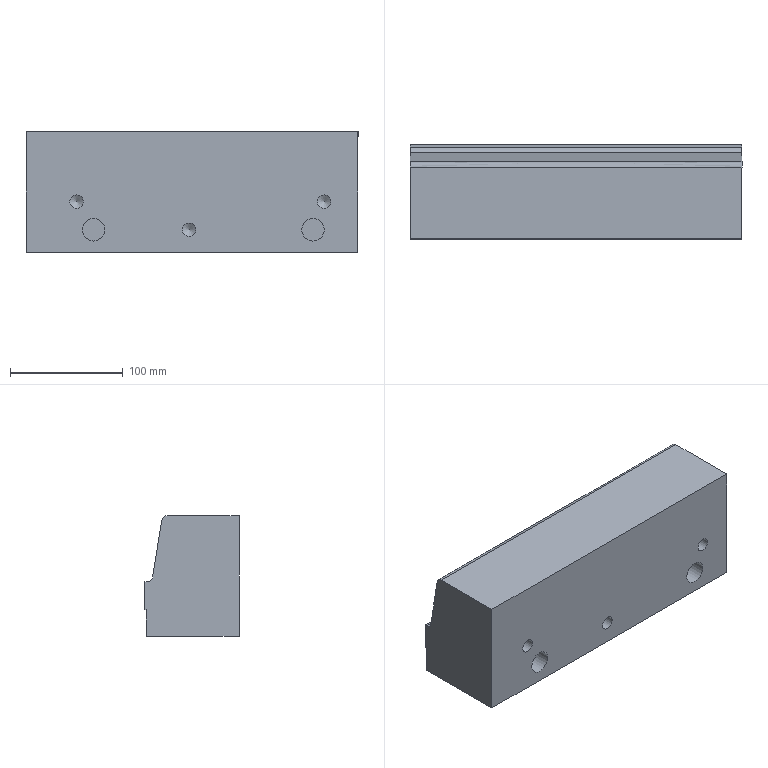Part | NX | features solid 2 | 1 solid | 22 faces | box 295 x 83.706 x 107.133 mm | volume 2418413 mm3 | plane 9 | cylinder 6 | spline 4 | cone 3 | commonest cylinder face diameters 12 x3 20 x2 10 x1
STEP:
#1=CARTESIAN_POINT('',(75.,-77.708,-50.));
#2=VERTEX_POINT('',#1);
#3=CARTESIAN_POINT('',(370.,-77.709,-50.));
#4=VERTEX_POINT('',#3);
#5=CARTESIAN_POINT('',(75.,-77.708,-50.));
#6=CARTESIAN_POINT('',(173.333,-77.71,-50.));
#7=CARTESIAN_POINT('',(271.667,-77.709,-50.));
#8=CARTESIAN_POINT('',(370.,-77.709,-50.));
#9=B_SPLINE_CURVE_WITH_KNOTS('',3,(#5,#6,#7,#8),.UNSPECIFIED.,.F.,.F.,(4,4),(0.1723,0.4673),.UNSPECIFIED.);
#10=EDGE_CURVE('',#2,#4,#9,.T.);
#11=ORIENTED_EDGE('',*,*,#10,.F.);
#12=CARTESIAN_POINT('',(75.,-77.507,-26.5));
#13=VERTEX_POINT('',#12);
#14=CARTESIAN_POINT('',(75.,-77.608,-38.267));
#15=DIRECTION('',(0.,-0.008536,-1.));
#16=VECTOR('',#15,1000.);
#17=LINE('',#14,#16);
#18=EDGE_CURVE('',#2,#13,#17,.F.);
#19=ORIENTED_EDGE('',*,*,#18,.T.);
#20=CARTESIAN_POINT('',(370.,-77.508,-26.5));
#21=VERTEX_POINT('',#20);
#22=CARTESIAN_POINT('',(75.,-77.507,-26.5));
#23=CARTESIAN_POINT('',(173.333,-77.509,-26.5));
#24=CARTESIAN_POINT('',(271.667,-77.508,-26.5));
#25=CARTESIAN_POINT('',(370.,-77.508,-26.5));
#26=B_SPLINE_CURVE_WITH_KNOTS('',3,(#22,#23,#24,#25),.UNSPECIFIED.,.F.,.F.,(4,4),(0.1378,0.4328),.UNSPECIFIED.);
#27=EDGE_CURVE('',#13,#21,#26,.T.);
#28=ORIENTED_EDGE('',*,*,#27,.T.);
#29=CARTESIAN_POINT('',(370.,-77.608,-38.267));
#30=DIRECTION('',(0.,-0.008536,-1.));
#31=VECTOR('',#30,1000.);
#32=LINE('',#29,#31);
#33=EDGE_CURVE('',#4,#21,#32,.F.);
#34=ORIENTED_EDGE('',*,*,#33,.F.);
#35=EDGE_LOOP('',(#11,#19,#28,#34));
#36=FACE_BOUND('',#35,.T.);
#37=CARTESIAN_POINT('',(75.,-77.507,-26.5));
#38=CARTESIAN_POINT('',(75.,-77.708,-50.));
#39=CARTESIAN_POINT('',(173.333,-77.509,-26.5));
#40=CARTESIAN_POINT('',(173.333,-77.71,-50.));
#41=CARTESIAN_POINT('',(271.667,-77.508,-26.5));
#42=CARTESIAN_POINT('',(271.667,-77.709,-50.));
#43=CARTESIAN_POINT('',(370.,-77.508,-26.5));
#44=CARTESIAN_POINT('',(370.,-77.709,-50.));
#45=B_SPLINE_SURFACE_WITH_KNOTS('',3,1,((#37,#38),(#39,#40),(#41,#42),(#43,#44)),.SURF_OF_LINEAR_EXTRUSION.,.F.,.F.,.F.,(4,4),(2,2),(0.5716,0.7876),(0.,1.),.PIECEWISE_BEZIER_KNOTS.);
#46=ADVANCED_FACE('',(#36),#45,.T.);
#47=ORIENTED_EDGE('',*,*,#33,.T.);
#48=CARTESIAN_POINT('',(370.,-76.295,-26.51));
#49=VERTEX_POINT('',#48);
#50=CARTESIAN_POINT('',(370.,-76.914,-26.505));
#51=DIRECTION('',(0.,-1.,0.008536));
#52=VECTOR('',#51,1000.);
#53=LINE('',#50,#52);
#54=EDGE_CURVE('',#49,#21,#53,.T.);
#55=ORIENTED_EDGE('',*,*,#54,.F.);
#56=CARTESIAN_POINT('',(370.,-76.295,-1.509));
#57=VERTEX_POINT('',#56);
#58=CARTESIAN_POINT('',(370.,-76.295,-14.009));
#59=DIRECTION('',(0.,0.,-1.));
#60=VECTOR('',#59,1000.);
#61=LINE('',#58,#60);
#62=EDGE_CURVE('',#57,#49,#61,.T.);
#63=ORIENTED_EDGE('',*,*,#62,.F.);
#64=CARTESIAN_POINT('',(370.,-78.294,-1.492));
#65=VERTEX_POINT('',#64);
#66=CARTESIAN_POINT('',(370.,46.797,-2.56));
#67=DIRECTION('',(0.,1.,-0.008536));
#68=VECTOR('',#67,1000.);
#69=LINE('',#66,#68);
#70=EDGE_CURVE('',#65,#57,#69,.T.);
#71=ORIENTED_EDGE('',*,*,#70,.F.);
#72=CARTESIAN_POINT('',(370.,-83.189,2.72));
#73=VERTEX_POINT('',#72);
#74=CARTESIAN_POINT('',(370.,-78.252,3.508));
#75=DIRECTION('',(-1.,0.,0.));
#76=DIRECTION('',(0.,0.,1.));
#77=AXIS2_PLACEMENT_3D('',#74,#75,#76);
#78=CIRCLE('',#77,5.);
#79=EDGE_CURVE('',#73,#65,#78,.F.);
#80=ORIENTED_EDGE('',*,*,#79,.F.);
#81=CARTESIAN_POINT('',(370.,-91.197,52.92));
#82=VERTEX_POINT('',#81);
#83=CARTESIAN_POINT('',(370.,-87.499,29.736));
#84=DIRECTION('',(0.,0.1575,-0.9875));
#85=VECTOR('',#84,1000.);
#86=LINE('',#83,#85);
#87=EDGE_CURVE('',#82,#73,#86,.T.);
#88=ORIENTED_EDGE('',*,*,#87,.F.);
#89=CARTESIAN_POINT('',(370.,-96.134,57.133));
#90=VERTEX_POINT('',#89);
#91=CARTESIAN_POINT('',(370.,-96.134,52.133));
#92=DIRECTION('',(-1.,0.,0.));
#93=DIRECTION('',(0.,0.,1.));
#94=AXIS2_PLACEMENT_3D('',#91,#92,#93);
#95=CIRCLE('',#94,5.);
#96=EDGE_CURVE('',#82,#90,#95,.F.);
#97=ORIENTED_EDGE('',*,*,#96,.T.);
#98=CARTESIAN_POINT('',(370.,-160.,57.133));
#99=VERTEX_POINT('',#98);
#100=CARTESIAN_POINT('',(370.,-91.869,57.133));
#101=DIRECTION('',(0.,-1.,0.));
#102=VECTOR('',#101,1000.);
#103=LINE('',#100,#102);
#104=EDGE_CURVE('',#90,#99,#103,.T.);
#105=ORIENTED_EDGE('',*,*,#104,.T.);
#106=CARTESIAN_POINT('',(370.,-160.,-50.));
#107=VERTEX_POINT('',#106);
#108=CARTESIAN_POINT('',(370.,-160.,200.));
#109=DIRECTION('',(0.,0.,1.));
#110=VECTOR('',#109,1000.);
#111=LINE('',#108,#110);
#112=EDGE_CURVE('',#107,#99,#111,.T.);
#113=ORIENTED_EDGE('',*,*,#112,.F.);
#114=CARTESIAN_POINT('',(370.,360.,-50.));
#115=DIRECTION('',(0.,-1.,0.));
#116=VECTOR('',#115,1000.);
#117=LINE('',#114,#116);
#118=EDGE_CURVE('',#107,#4,#117,.F.);
#119=ORIENTED_EDGE('',*,*,#118,.T.);
#120=EDGE_LOOP('',(#47,#55,#63,#71,#80,#88,#97,#105,#113,#119));
#121=FACE_BOUND('',#120,.T.);
#122=CARTESIAN_POINT('',(370.,360.,0.));
#123=DIRECTION('',(-1.,0.,0.));
#124=DIRECTION('',(0.,0.,1.));
#125=AXIS2_PLACEMENT_3D('',#122,#123,#124);
#126=PLANE('',#125);
#127=ADVANCED_FACE('',(#121),#126,.F.);
#128=CARTESIAN_POINT('',(75.,-160.,-50.));
#129=VERTEX_POINT('',#128);
#130=CARTESIAN_POINT('',(75.,-160.,-50.));
#131=DIRECTION('',(0.,1.,0.));
#132=VECTOR('',#131,1000.);
#133=LINE('',#130,#132);
#134=EDGE_CURVE('',#129,#2,#133,.T.);
#135=ORIENTED_EDGE('',*,*,#134,.T.);
#136=ORIENTED_EDGE('',*,*,#10,.T.);
#137=ORIENTED_EDGE('',*,*,#118,.F.);
#138=CARTESIAN_POINT('',(-571.479,-160.,-50.));
#139=DIRECTION('',(1.,0.,0.));
#140=VECTOR('',#139,1000.);
#141=LINE('',#138,#140);
#142=EDGE_CURVE('',#129,#107,#141,.T.);
#143=ORIENTED_EDGE('',*,*,#142,.F.);
#144=EDGE_LOOP('',(#135,#136,#137,#143));
#145=FACE_BOUND('',#144,.T.);
#146=CARTESIAN_POINT('',(-571.479,-75.471,-50.));
#147=DIRECTION('',(0.,0.,-1.));
#148=DIRECTION('',(-1.,0.,0.));
#149=AXIS2_PLACEMENT_3D('',#146,#147,#148);
#150=PLANE('',#149);
#151=ADVANCED_FACE('',(#145),#150,.T.);
#152=ORIENTED_EDGE('',*,*,#142,.T.);
#153=ORIENTED_EDGE('',*,*,#112,.T.);
#154=CARTESIAN_POINT('',(75.,-160.,57.133));
#155=VERTEX_POINT('',#154);
#156=CARTESIAN_POINT('',(-705.,-160.,57.133));
#157=DIRECTION('',(1.,0.,0.));
#158=VECTOR('',#157,1000.);
#159=LINE('',#156,#158);
#160=EDGE_CURVE('',#155,#99,#159,.T.);
#161=ORIENTED_EDGE('',*,*,#160,.F.);
#162=CARTESIAN_POINT('',(75.,-160.,200.));
#163=DIRECTION('',(0.,0.,1.));
#164=VECTOR('',#163,1000.);
#165=LINE('',#162,#164);
#166=EDGE_CURVE('',#129,#155,#165,.T.);
#167=ORIENTED_EDGE('',*,*,#166,.F.);
#168=EDGE_LOOP('',(#152,#153,#161,#167));
#169=FACE_BOUND('',#168,.T.);
#170=CARTESIAN_POINT('',(340.,-160.,1.));
#171=VERTEX_POINT('',#170);
#172=CARTESIAN_POINT('',(340.,-160.,-5.));
#173=DIRECTION('',(0.,1.,0.));
#174=DIRECTION('',(0.,0.,1.));
#175=AXIS2_PLACEMENT_3D('',#172,#173,#174);
#176=CIRCLE('',#175,6.);
#177=EDGE_CURVE('',#171,#171,#176,.T.);
#178=ORIENTED_EDGE('',*,*,#177,.T.);
#179=EDGE_LOOP('',(#178));
#180=FACE_BOUND('',#179,.T.);
#181=CARTESIAN_POINT('',(220.,-160.,-24.));
#182=VERTEX_POINT('',#181);
#183=CARTESIAN_POINT('',(220.,-160.,-30.));
#184=DIRECTION('',(0.,1.,0.));
#185=DIRECTION('',(0.,0.,1.));
#186=AXIS2_PLACEMENT_3D('',#183,#184,#185);
#187=CIRCLE('',#186,6.);
#188=EDGE_CURVE('',#182,#182,#187,.T.);
#189=ORIENTED_EDGE('',*,*,#188,.T.);
#190=EDGE_LOOP('',(#189));
#191=FACE_BOUND('',#190,.T.);
#192=CARTESIAN_POINT('',(120.,-160.,1.));
#193=VERTEX_POINT('',#192);
#194=CARTESIAN_POINT('',(120.,-160.,-5.));
#195=DIRECTION('',(0.,1.,0.));
#196=DIRECTION('',(0.,0.,1.));
#197=AXIS2_PLACEMENT_3D('',#194,#195,#196);
#198=CIRCLE('',#197,6.);
#199=EDGE_CURVE('',#193,#193,#198,.T.);
#200=ORIENTED_EDGE('',*,*,#199,.T.);
#201=EDGE_LOOP('',(#200));
#202=FACE_BOUND('',#201,.T.);
#203=CARTESIAN_POINT('',(330.,-160.,-20.));
#204=VERTEX_POINT('',#203);
#205=CARTESIAN_POINT('',(330.,-160.,-30.));
#206=DIRECTION('',(0.,1.,0.));
#207=DIRECTION('',(0.,0.,1.));
#208=AXIS2_PLACEMENT_3D('',#205,#206,#207);
#209=CIRCLE('',#208,10.);
#210=EDGE_CURVE('',#204,#204,#209,.T.);
#211=ORIENTED_EDGE('',*,*,#210,.T.);
#212=EDGE_LOOP('',(#211));
#213=FACE_BOUND('',#212,.T.);
#214=CARTESIAN_POINT('',(135.,-160.,-20.));
#215=VERTEX_POINT('',#214);
#216=CARTESIAN_POINT('',(135.,-160.,-30.));
#217=DIRECTION('',(0.,1.,0.));
#218=DIRECTION('',(0.,0.,1.));
#219=AXIS2_PLACEMENT_3D('',#216,#217,#218);
#220=CIRCLE('',#219,10.);
#221=EDGE_CURVE('',#215,#215,#220,.T.);
#222=ORIENTED_EDGE('',*,*,#221,.T.);
#223=EDGE_LOOP('',(#222));
#224=FACE_BOUND('',#223,.T.);
#225=CARTESIAN_POINT('',(-705.,-160.,200.));
#226=DIRECTION('',(0.,1.,0.));
#227=DIRECTION('',(0.,0.,1.));
#228=AXIS2_PLACEMENT_3D('',#225,#226,#227);
#229=PLANE('',#228);
#230=ADVANCED_FACE('',(#169,#180,#191,#202,#213,#224),#229,.F.);
#231=ORIENTED_EDGE('',*,*,#96,.F.);
#232=CARTESIAN_POINT('',(75.,-91.197,52.92));
#233=VERTEX_POINT('',#232);
#234=CARTESIAN_POINT('',(75.,-91.197,52.92));
#235=CARTESIAN_POINT('',(173.333,-91.197,52.92));
#236=CARTESIAN_POINT('',(271.667,-91.197,52.92));
#237=CARTESIAN_POINT('',(370.,-91.197,52.92));
#238=B_SPLINE_CURVE_WITH_KNOTS('',3,(#234,#235,#236,#237),.UNSPECIFIED.,.F.,.F.,(4,4),(0.2731,0.5681),.UNSPECIFIED.);
#239=EDGE_CURVE('',#233,#82,#238,.T.);
#240=ORIENTED_EDGE('',*,*,#239,.F.);
#241=CARTESIAN_POINT('',(75.,-96.134,57.133));
#242=VERTEX_POINT('',#241);
#243=CARTESIAN_POINT('',(75.,-96.134,52.133));
#244=DIRECTION('',(-1.,0.,0.));
#245=DIRECTION('',(0.,0.,1.));
#246=AXIS2_PLACEMENT_3D('',#243,#244,#245);
#247=CIRCLE('',#246,5.);
#248=EDGE_CURVE('',#233,#242,#247,.F.);
#249=ORIENTED_EDGE('',*,*,#248,.T.);
#250=CARTESIAN_POINT('',(370.,-96.134,57.133));
#251=CARTESIAN_POINT('',(271.667,-96.134,57.133));
#252=CARTESIAN_POINT('',(173.333,-96.134,57.133));
#253=CARTESIAN_POINT('',(75.,-96.134,57.133));
#254=B_SPLINE_CURVE_WITH_KNOTS('',3,(#250,#251,#252,#253),.UNSPECIFIED.,.F.,.F.,(4,4),(0.3736,0.6686),.UNSPECIFIED.);
#255=EDGE_CURVE('',#90,#242,#254,.T.);
#256=ORIENTED_EDGE('',*,*,#255,.F.);
#257=EDGE_LOOP('',(#231,#240,#249,#256));
#258=FACE_BOUND('',#257,.T.);
#259=CARTESIAN_POINT('',(370.,-91.197,52.92));
#260=CARTESIAN_POINT('',(370.,-91.869,57.133));
#261=CARTESIAN_POINT('',(370.,-96.134,57.133));
#262=CARTESIAN_POINT('',(271.667,-91.197,52.92));
#263=CARTESIAN_POINT('',(271.667,-91.869,57.133));
#264=CARTESIAN_POINT('',(271.667,-96.134,57.133));
#265=CARTESIAN_POINT('',(173.333,-91.197,52.92));
#266=CARTESIAN_POINT('',(173.333,-91.869,57.133));
#267=CARTESIAN_POINT('',(173.333,-96.134,57.133));
#268=CARTESIAN_POINT('',(75.,-91.197,52.92));
#269=CARTESIAN_POINT('',(75.,-91.869,57.133));
#270=CARTESIAN_POINT('',(75.,-96.134,57.133));
#271=(BOUNDED_SURFACE()B_SPLINE_SURFACE(3,2,((#259,#260,#261),(#262,#263,#264),(#265,#266,#267),(#268,#269,#270)),.UNSPECIFIED.,.F.,.F.,.F.)B_SPLINE_SURFACE_WITH_KNOTS((4,4),(3,3),(0.4893,0.7843),(0.,1.),.PIECEWISE_BEZIER_KNOTS.)GEOMETRIC_REPRESENTATION_ITEM()RATIONAL_B_SPLINE_SURFACE(((1.,0.7608,1.),(1.,0.7608,1.),(1.,0.7608,1.),(1.,0.7608,1.)))REPRESENTATION_ITEM('')SURFACE());
#272=ADVANCED_FACE('',(#258),#271,.T.);
#273=ORIENTED_EDGE('',*,*,#239,.T.);
#274=ORIENTED_EDGE('',*,*,#87,.T.);
#275=CARTESIAN_POINT('',(75.,-83.189,2.72));
#276=VERTEX_POINT('',#275);
#277=CARTESIAN_POINT('',(75.,-83.189,2.72));
#278=CARTESIAN_POINT('',(173.333,-83.189,2.72));
#279=CARTESIAN_POINT('',(271.667,-83.189,2.72));
#280=CARTESIAN_POINT('',(370.,-83.189,2.72));
#281=B_SPLINE_CURVE_WITH_KNOTS('',3,(#277,#278,#279,#280),.UNSPECIFIED.,.F.,.F.,(4,4),(0.3113,0.6615),.UNSPECIFIED.);
#282=EDGE_CURVE('',#276,#73,#281,.T.);
#283=ORIENTED_EDGE('',*,*,#282,.F.);
#284=CARTESIAN_POINT('',(75.,-87.499,29.736));
#285=DIRECTION('',(0.,0.1575,-0.9875));
#286=VECTOR('',#285,1000.);
#287=LINE('',#284,#286);
#288=EDGE_CURVE('',#233,#276,#287,.T.);
#289=ORIENTED_EDGE('',*,*,#288,.F.);
#290=EDGE_LOOP('',(#273,#274,#283,#289));
#291=FACE_BOUND('',#290,.T.);
#292=CARTESIAN_POINT('',(808.196,-82.695,-0.3814));
#293=CARTESIAN_POINT('',(-199.284,-82.695,-0.3814));
#294=CARTESIAN_POINT('',(808.196,-92.303,59.853));
#295=CARTESIAN_POINT('',(-199.284,-92.303,59.853));
#296=B_SPLINE_SURFACE_WITH_KNOTS('',1,1,((#292,#293),(#294,#295)),.PLANE_SURF.,.F.,.F.,.F.,(2,2),(2,2),(-0.06964,1.283),(-0.1722,1.),.UNSPECIFIED.);
#297=ADVANCED_FACE('',(#291),#296,.F.);
#298=ORIENTED_EDGE('',*,*,#282,.T.);
#299=ORIENTED_EDGE('',*,*,#79,.T.);
#300=CARTESIAN_POINT('',(75.,-78.294,-1.492));
#301=VERTEX_POINT('',#300);
#302=CARTESIAN_POINT('',(370.,-78.294,-1.492));
#303=CARTESIAN_POINT('',(271.667,-78.294,-1.492));
#304=CARTESIAN_POINT('',(173.333,-78.294,-1.492));
#305=CARTESIAN_POINT('',(75.,-78.294,-1.492));
#306=B_SPLINE_CURVE_WITH_KNOTS('',3,(#302,#303,#304,#305),.UNSPECIFIED.,.F.,.F.,(4,4),(0.3388,0.6888),.UNSPECIFIED.);
#307=EDGE_CURVE('',#65,#301,#306,.T.);
#308=ORIENTED_EDGE('',*,*,#307,.T.);
#309=CARTESIAN_POINT('',(75.,-78.252,3.508));
#310=DIRECTION('',(-1.,0.,0.));
#311=DIRECTION('',(0.,0.,1.));
#312=AXIS2_PLACEMENT_3D('',#309,#310,#311);
#313=CIRCLE('',#312,5.);
#314=EDGE_CURVE('',#276,#301,#313,.F.);
#315=ORIENTED_EDGE('',*,*,#314,.F.);
#316=EDGE_LOOP('',(#298,#299,#308,#315));
#317=FACE_BOUND('',#316,.T.);
#318=CARTESIAN_POINT('',(6000655.556,-78.252,3.508));
#319=DIRECTION('',(-1.,0.,0.));
#320=DIRECTION('',(0.,-0.1575,0.9875));
#321=AXIS2_PLACEMENT_3D('',#318,#319,#320);
#322=CYLINDRICAL_SURFACE('',#321,5.);
#323=ADVANCED_FACE('',(#317),#322,.F.);
#324=ORIENTED_EDGE('',*,*,#307,.F.);
#325=ORIENTED_EDGE('',*,*,#70,.T.);
#326=CARTESIAN_POINT('',(75.,-76.294,-1.509));
#327=VERTEX_POINT('',#326);
#328=CARTESIAN_POINT('',(75.,-76.294,-1.509));
#329=CARTESIAN_POINT('',(173.333,-76.295,-1.509));
#330=CARTESIAN_POINT('',(271.667,-76.295,-1.509));
#331=CARTESIAN_POINT('',(370.,-76.295,-1.509));
#332=B_SPLINE_CURVE_WITH_KNOTS('',3,(#328,#329,#330,#331),.UNSPECIFIED.,.F.,.F.,(4,4),(0.4725,0.7675),.UNSPECIFIED.);
#333=EDGE_CURVE('',#327,#57,#332,.T.);
#334=ORIENTED_EDGE('',*,*,#333,.F.);
#335=CARTESIAN_POINT('',(75.,46.797,-2.56));
#336=DIRECTION('',(0.,1.,-0.008536));
#337=VECTOR('',#336,1000.);
#338=LINE('',#335,#337);
#339=EDGE_CURVE('',#301,#327,#338,.T.);
#340=ORIENTED_EDGE('',*,*,#339,.F.);
#341=EDGE_LOOP('',(#324,#325,#334,#340));
#342=FACE_BOUND('',#341,.T.);
#343=CARTESIAN_POINT('',(35.495,46.797,-2.56));
#344=DIRECTION('',(0.,-0.008536,-1.));
#345=DIRECTION('',(0.,-1.,0.008536));
#346=AXIS2_PLACEMENT_3D('',#343,#344,#345);
#347=PLANE('',#346);
#348=ADVANCED_FACE('',(#342),#347,.F.);
#349=ORIENTED_EDGE('',*,*,#333,.T.);
#350=ORIENTED_EDGE('',*,*,#62,.T.);
#351=CARTESIAN_POINT('',(75.,-76.294,-26.51));
#352=VERTEX_POINT('',#351);
#353=CARTESIAN_POINT('',(370.,-76.295,-26.51));
#354=CARTESIAN_POINT('',(271.667,-76.295,-26.51));
#355=CARTESIAN_POINT('',(173.333,-76.295,-26.51));
#356=CARTESIAN_POINT('',(75.,-76.294,-26.51));
#357=B_SPLINE_CURVE_WITH_KNOTS('',3,(#353,#354,#355,#356),.UNSPECIFIED.,.F.,.F.,(4,4),(0.29,0.585),.UNSPECIFIED.);
#358=EDGE_CURVE('',#49,#352,#357,.T.);
#359=ORIENTED_EDGE('',*,*,#358,.T.);
#360=CARTESIAN_POINT('',(75.,-76.294,-14.008));
#361=DIRECTION('',(0.,0.,-1.));
#362=VECTOR('',#361,1000.);
#363=LINE('',#360,#362);
#364=EDGE_CURVE('',#327,#352,#363,.T.);
#365=ORIENTED_EDGE('',*,*,#364,.F.);
#366=EDGE_LOOP('',(#349,#350,#359,#365));
#367=FACE_BOUND('',#366,.T.);
#368=CARTESIAN_POINT('',(370.,-76.295,-1.509));
#369=CARTESIAN_POINT('',(370.,-76.295,-26.51));
#370=CARTESIAN_POINT('',(271.667,-76.295,-1.509));
#371=CARTESIAN_POINT('',(271.667,-76.295,-26.51));
#372=CARTESIAN_POINT('',(173.333,-76.295,-1.509));
#373=CARTESIAN_POINT('',(173.333,-76.295,-26.51));
#374=CARTESIAN_POINT('',(75.,-76.294,-1.509));
#375=CARTESIAN_POINT('',(75.,-76.294,-26.51));
#376=B_SPLINE_SURFACE_WITH_KNOTS('',3,1,((#368,#369),(#370,#371),(#372,#373),(#374,#375)),.SURF_OF_LINEAR_EXTRUSION.,.F.,.F.,.F.,(4,4),(2,2),(0.2124,0.4284),(0.,1.),.PIECEWISE_BEZIER_KNOTS.);
#377=ADVANCED_FACE('',(#367),#376,.F.);
#378=ORIENTED_EDGE('',*,*,#27,.F.);
#379=CARTESIAN_POINT('',(75.,-76.914,-26.505));
#380=DIRECTION('',(0.,-1.,0.008536));
#381=VECTOR('',#380,1000.);
#382=LINE('',#379,#381);
#383=EDGE_CURVE('',#352,#13,#382,.T.);
#384=ORIENTED_EDGE('',*,*,#383,.F.);
#385=ORIENTED_EDGE('',*,*,#358,.F.);
#386=ORIENTED_EDGE('',*,*,#54,.T.);
#387=EDGE_LOOP('',(#378,#384,#385,#386));
#388=FACE_BOUND('',#387,.T.);
#389=CARTESIAN_POINT('',(-437.652,-76.914,-26.505));
#390=DIRECTION('',(0.,0.008536,1.));
#391=DIRECTION('',(0.,-1.,0.008536));
#392=AXIS2_PLACEMENT_3D('',#389,#390,#391);
#393=PLANE('',#392);
#394=ADVANCED_FACE('',(#388),#393,.F.);
#395=ORIENTED_EDGE('',*,*,#383,.T.);
#396=ORIENTED_EDGE('',*,*,#18,.F.);
#397=ORIENTED_EDGE('',*,*,#134,.F.);
#398=ORIENTED_EDGE('',*,*,#166,.T.);
#399=CARTESIAN_POINT('',(75.,-91.869,57.133));
#400=DIRECTION('',(0.,-1.,0.));
#401=VECTOR('',#400,1000.);
#402=LINE('',#399,#401);
#403=EDGE_CURVE('',#242,#155,#402,.T.);
#404=ORIENTED_EDGE('',*,*,#403,.F.);
#405=ORIENTED_EDGE('',*,*,#248,.F.);
#406=ORIENTED_EDGE('',*,*,#288,.T.);
#407=ORIENTED_EDGE('',*,*,#314,.T.);
#408=ORIENTED_EDGE('',*,*,#339,.T.);
#409=ORIENTED_EDGE('',*,*,#364,.T.);
#410=EDGE_LOOP('',(#395,#396,#397,#398,#404,#405,#406,#407,#408,#409));
#411=FACE_BOUND('',#410,.T.);
#412=CARTESIAN_POINT('',(75.,360.,0.));
#413=DIRECTION('',(-1.,0.,0.));
#414=DIRECTION('',(0.,0.,1.));
#415=AXIS2_PLACEMENT_3D('',#412,#413,#414);
#416=PLANE('',#415);
#417=ADVANCED_FACE('',(#411),#416,.T.);
#418=ORIENTED_EDGE('',*,*,#104,.F.);
#419=ORIENTED_EDGE('',*,*,#255,.T.);
#420=ORIENTED_EDGE('',*,*,#403,.T.);
#421=ORIENTED_EDGE('',*,*,#160,.T.);
#422=EDGE_LOOP('',(#418,#419,#420,#421));
#423=FACE_BOUND('',#422,.T.);
#424=CARTESIAN_POINT('',(743.607,-91.869,57.133));
#425=DIRECTION('',(0.,0.,1.));
#426=DIRECTION('',(1.,0.,0.));
#427=AXIS2_PLACEMENT_3D('',#424,#425,#426);
#428=PLANE('',#427);
#429=ADVANCED_FACE('',(#423),#428,.T.);
#430=CARTESIAN_POINT('',(340.,-130.,1.));
#431=VERTEX_POINT('',#430);
#432=CARTESIAN_POINT('',(340.,-130.,-5.));
#433=DIRECTION('',(0.,1.,0.));
#434=DIRECTION('',(0.,0.,1.));
#435=AXIS2_PLACEMENT_3D('',#432,#433,#434);
#436=CIRCLE('',#435,6.);
#437=EDGE_CURVE('',#431,#431,#436,.T.);
#438=ORIENTED_EDGE('',*,*,#437,.F.);
#439=EDGE_LOOP('',(#438));
#440=FACE_BOUND('',#439,.T.);
#441=CARTESIAN_POINT('',(340.,-126.395,-5.));
#442=VERTEX_POINT('',#441);
#443=VERTEX_LOOP('',#442);
#444=FACE_BOUND('',#443,.T.);
#445=CARTESIAN_POINT('',(340.,-130.,-5.));
#446=DIRECTION('',(0.,-1.,0.));
#447=DIRECTION('',(0.,0.,-1.));
#448=AXIS2_PLACEMENT_3D('',#445,#446,#447);
#449=CONICAL_SURFACE('',#448,6.,1.03);
#450=ADVANCED_FACE('',(#440,#444),#449,.F.);
#451=ORIENTED_EDGE('',*,*,#437,.T.);
#452=EDGE_LOOP('',(#451));
#453=FACE_BOUND('',#452,.T.);
#454=ORIENTED_EDGE('',*,*,#177,.F.);
#455=EDGE_LOOP('',(#454));
#456=FACE_BOUND('',#455,.T.);
#457=CARTESIAN_POINT('',(340.,-160.,-5.));
#458=DIRECTION('',(0.,1.,0.));
#459=DIRECTION('',(0.,0.,1.));
#460=AXIS2_PLACEMENT_3D('',#457,#458,#459);
#461=CYLINDRICAL_SURFACE('',#460,6.);
#462=ADVANCED_FACE('',(#453,#456),#461,.F.);
#463=CARTESIAN_POINT('',(220.,-130.,-24.));
#464=VERTEX_POINT('',#463);
#465=CARTESIAN_POINT('',(220.,-130.,-30.));
#466=DIRECTION('',(0.,1.,0.));
#467=DIRECTION('',(0.,0.,1.));
#468=AXIS2_PLACEMENT_3D('',#465,#466,#467);
#469=CIRCLE('',#468,6.);
#470=EDGE_CURVE('',#464,#464,#469,.T.);
#471=ORIENTED_EDGE('',*,*,#470,.F.);
#472=EDGE_LOOP('',(#471));
#473=FACE_BOUND('',#472,.T.);
#474=CARTESIAN_POINT('',(220.,-126.395,-30.));
#475=VERTEX_POINT('',#474);
#476=VERTEX_LOOP('',#475);
#477=FACE_BOUND('',#476,.T.);
#478=CARTESIAN_POINT('',(220.,-130.,-30.));
#479=DIRECTION('',(0.,-1.,0.));
#480=DIRECTION('',(0.,0.,-1.));
#481=AXIS2_PLACEMENT_3D('',#478,#479,#480);
#482=CONICAL_SURFACE('',#481,6.,1.03);
#483=ADVANCED_FACE('',(#473,#477),#482,.F.);
#484=ORIENTED_EDGE('',*,*,#470,.T.);
#485=EDGE_LOOP('',(#484));
#486=FACE_BOUND('',#485,.T.);
#487=ORIENTED_EDGE('',*,*,#188,.F.);
#488=EDGE_LOOP('',(#487));
#489=FACE_BOUND('',#488,.T.);
#490=CARTESIAN_POINT('',(220.,-160.,-30.));
#491=DIRECTION('',(0.,1.,0.));
#492=DIRECTION('',(0.,0.,1.));
#493=AXIS2_PLACEMENT_3D('',#490,#491,#492);
#494=CYLINDRICAL_SURFACE('',#493,6.);
#495=ADVANCED_FACE('',(#486,#489),#494,.F.);
#496=CARTESIAN_POINT('',(120.,-130.,1.));
#497=VERTEX_POINT('',#496);
#498=CARTESIAN_POINT('',(120.,-130.,-5.));
#499=DIRECTION('',(0.,1.,0.));
#500=DIRECTION('',(0.,0.,1.));
#501=AXIS2_PLACEMENT_3D('',#498,#499,#500);
#502=CIRCLE('',#501,6.);
#503=EDGE_CURVE('',#497,#497,#502,.T.);
#504=ORIENTED_EDGE('',*,*,#503,.F.);
#505=EDGE_LOOP('',(#504));
#506=FACE_BOUND('',#505,.T.);
#507=CARTESIAN_POINT('',(120.,-126.395,-5.));
#508=VERTEX_POINT('',#507);
#509=VERTEX_LOOP('',#508);
#510=FACE_BOUND('',#509,.T.);
#511=CARTESIAN_POINT('',(120.,-130.,-5.));
#512=DIRECTION('',(0.,-1.,0.));
#513=DIRECTION('',(0.,0.,-1.));
#514=AXIS2_PLACEMENT_3D('',#511,#512,#513);
#515=CONICAL_SURFACE('',#514,6.,1.03);
#516=ADVANCED_FACE('',(#506,#510),#515,.F.);
#517=ORIENTED_EDGE('',*,*,#503,.T.);
#518=EDGE_LOOP('',(#517));
#519=FACE_BOUND('',#518,.T.);
#520=ORIENTED_EDGE('',*,*,#199,.F.);
#521=EDGE_LOOP('',(#520));
#522=FACE_BOUND('',#521,.T.);
#523=CARTESIAN_POINT('',(120.,-160.,-5.));
#524=DIRECTION('',(0.,1.,0.));
#525=DIRECTION('',(0.,0.,1.));
#526=AXIS2_PLACEMENT_3D('',#523,#524,#525);
#527=CYLINDRICAL_SURFACE('',#526,6.);
#528=ADVANCED_FACE('',(#519,#522),#527,.F.);
#529=CARTESIAN_POINT('',(330.,-130.,-20.));
#530=VERTEX_POINT('',#529);
#531=CARTESIAN_POINT('',(330.,-130.,-30.));
#532=DIRECTION('',(0.,1.,0.));
#533=DIRECTION('',(0.,0.,1.));
#534=AXIS2_PLACEMENT_3D('',#531,#532,#533);
#535=CIRCLE('',#534,10.);
#536=EDGE_CURVE('',#530,#530,#535,.T.);
#537=ORIENTED_EDGE('',*,*,#536,.T.);
#538=EDGE_LOOP('',(#537));
#539=FACE_BOUND('',#538,.T.);
#540=ORIENTED_EDGE('',*,*,#210,.F.);
#541=EDGE_LOOP('',(#540));
#542=FACE_BOUND('',#541,.T.);
#543=CARTESIAN_POINT('',(330.,-160.,-30.));
#544=DIRECTION('',(0.,1.,0.));
#545=DIRECTION('',(0.,0.,1.));
#546=AXIS2_PLACEMENT_3D('',#543,#544,#545);
#547=CYLINDRICAL_SURFACE('',#546,10.);
#548=ADVANCED_FACE('',(#539,#542),#547,.F.);
#549=ORIENTED_EDGE('',*,*,#536,.F.);
#550=EDGE_LOOP('',(#549));
#551=FACE_BOUND('',#550,.T.);
#552=CARTESIAN_POINT('',(330.,-130.,-30.));
#553=DIRECTION('',(0.,1.,0.));
#554=DIRECTION('',(0.,0.,1.));
#555=AXIS2_PLACEMENT_3D('',#552,#553,#554);
#556=PLANE('',#555);
#557=ADVANCED_FACE('',(#551),#556,.F.);
#558=CARTESIAN_POINT('',(135.,-130.,-20.));
#559=VERTEX_POINT('',#558);
#560=CARTESIAN_POINT('',(135.,-130.,-30.));
#561=DIRECTION('',(0.,1.,0.));
#562=DIRECTION('',(0.,0.,1.));
#563=AXIS2_PLACEMENT_3D('',#560,#561,#562);
#564=CIRCLE('',#563,10.);
#565=EDGE_CURVE('',#559,#559,#564,.T.);
#566=ORIENTED_EDGE('',*,*,#565,.T.);
#567=EDGE_LOOP('',(#566));
#568=FACE_BOUND('',#567,.T.);
#569=ORIENTED_EDGE('',*,*,#221,.F.);
#570=EDGE_LOOP('',(#569));
#571=FACE_BOUND('',#570,.T.);
#572=CARTESIAN_POINT('',(135.,-160.,-30.));
#573=DIRECTION('',(0.,1.,0.));
#574=DIRECTION('',(0.,0.,1.));
#575=AXIS2_PLACEMENT_3D('',#572,#573,#574);
#576=CYLINDRICAL_SURFACE('',#575,10.);
#577=ADVANCED_FACE('',(#568,#571),#576,.F.);
#578=ORIENTED_EDGE('',*,*,#565,.F.);
#579=EDGE_LOOP('',(#578));
#580=FACE_BOUND('',#579,.T.);
#581=CARTESIAN_POINT('',(135.,-130.,-30.));
#582=DIRECTION('',(0.,1.,0.));
#583=DIRECTION('',(0.,0.,1.));
#584=AXIS2_PLACEMENT_3D('',#581,#582,#583);
#585=PLANE('',#584);
#586=ADVANCED_FACE('',(#580),#585,.F.);
#587=CLOSED_SHELL('',(#46,#127,#151,#230,#272,#297,#323,#348,#377,#394,#417,#429,#450,#462,#483,#495,#516,#528,#548,#557,#577,#586));
#588=MANIFOLD_SOLID_BREP('',#587);
#589=(LENGTH_UNIT()NAMED_UNIT(*)SI_UNIT(.MILLI.,.METRE.));
#590=UNCERTAINTY_MEASURE_WITH_UNIT(LENGTH_MEASURE(0.0508),#589,'','');
#591=(NAMED_UNIT(*)PLANE_ANGLE_UNIT()SI_UNIT($,.RADIAN.));
#592=(NAMED_UNIT(*)SI_UNIT($,.STERADIAN.)SOLID_ANGLE_UNIT());
#593=(GEOMETRIC_REPRESENTATION_CONTEXT(3)GLOBAL_UNCERTAINTY_ASSIGNED_CONTEXT((#590))GLOBAL_UNIT_ASSIGNED_CONTEXT((#589,#591,#592))REPRESENTATION_CONTEXT('',''));
#594=ADVANCED_BREP_SHAPE_REPRESENTATION('',(#588),#593);